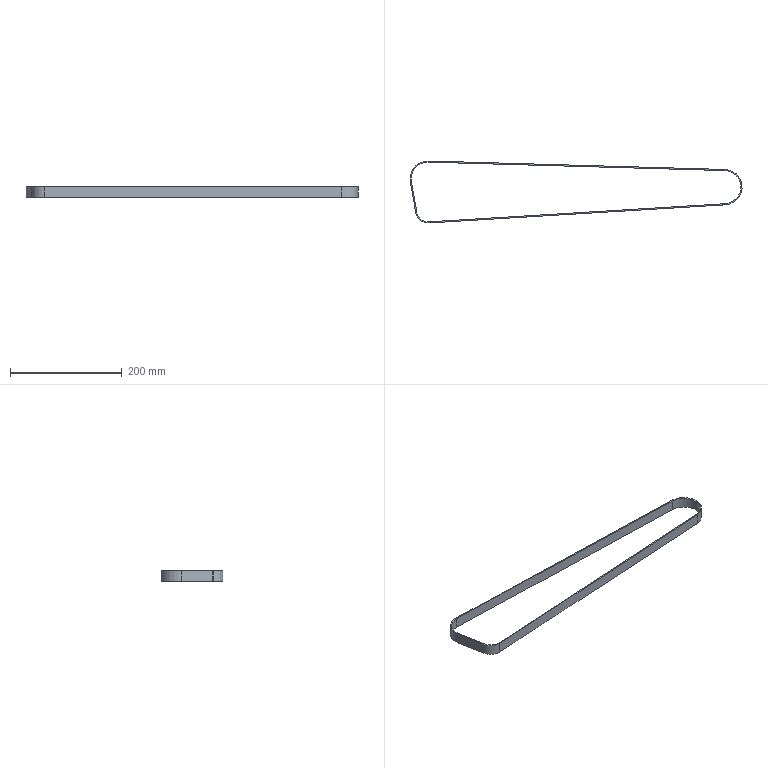Part | SolidWorks | features BaseBody 1 | 1 solid | 14 faces | box 593.838 x 110.876 x 19.05 mm | volume 50225 mm3 | plane 8 | cylinder 6 | commonest cylinder face diameters 59.266 x2 63.33 x2 39.054 x1 43.118 x1
STEP:
#1=CARTESIAN_POINT('',(532.317,-44.647,9.525));
#2=VERTEX_POINT('',#1);
#3=CARTESIAN_POINT('',(532.317,-44.647,-9.525));
#4=VERTEX_POINT('',#3);
#5=CARTESIAN_POINT('',(532.317,-44.647,9.525));
#6=DIRECTION('',(0.,0.,-1.));
#7=VECTOR('',#6,1000.);
#8=LINE('',#5,#7);
#9=EDGE_CURVE('',#2,#4,#8,.T.);
#10=ORIENTED_EDGE('',*,*,#9,.F.);
#11=CARTESIAN_POINT('',(531.349,14.552,9.525));
#12=VERTEX_POINT('',#11);
#13=CARTESIAN_POINT('',(530.507,-15.069,9.525));
#14=DIRECTION('',(0.,0.,-1.));
#15=DIRECTION('',(-0.06107,0.9981,0.));
#16=AXIS2_PLACEMENT_3D('',#13,#14,#15);
#17=CIRCLE('',#16,29.633);
#18=EDGE_CURVE('',#12,#2,#17,.T.);
#19=ORIENTED_EDGE('',*,*,#18,.F.);
#20=CARTESIAN_POINT('',(531.349,14.552,-9.525));
#21=VERTEX_POINT('',#20);
#22=CARTESIAN_POINT('',(531.349,14.552,9.525));
#23=DIRECTION('',(0.,0.,1.));
#24=VECTOR('',#23,1000.);
#25=LINE('',#22,#24);
#26=EDGE_CURVE('',#21,#12,#25,.T.);
#27=ORIENTED_EDGE('',*,*,#26,.F.);
#28=CARTESIAN_POINT('',(530.507,-15.069,-9.525));
#29=DIRECTION('',(0.,0.,-1.));
#30=DIRECTION('',(-0.06107,0.9981,0.));
#31=AXIS2_PLACEMENT_3D('',#28,#29,#30);
#32=CIRCLE('',#31,29.633);
#33=EDGE_CURVE('',#21,#4,#32,.T.);
#34=ORIENTED_EDGE('',*,*,#33,.T.);
#35=EDGE_LOOP('',(#10,#19,#27,#34));
#36=FACE_OUTER_BOUND('',#35,.T.);
#37=CARTESIAN_POINT('',(530.507,-15.069,0.));
#38=DIRECTION('',(0.,0.,1.));
#39=DIRECTION('',(-0.06107,0.9981,0.));
#40=AXIS2_PLACEMENT_3D('',#37,#38,#39);
#41=CYLINDRICAL_SURFACE('',#40,29.633);
#42=ADVANCED_FACE('',(#36),#41,.F.);
#43=CARTESIAN_POINT('',(532.441,-46.675,-9.525));
#44=VERTEX_POINT('',#43);
#45=CARTESIAN_POINT('',(532.441,-46.675,9.525));
#46=VERTEX_POINT('',#45);
#47=CARTESIAN_POINT('',(532.441,-46.675,-9.525));
#48=DIRECTION('',(0.,0.,1.));
#49=VECTOR('',#48,1000.);
#50=LINE('',#47,#49);
#51=EDGE_CURVE('',#44,#46,#50,.T.);
#52=ORIENTED_EDGE('',*,*,#51,.F.);
#53=CARTESIAN_POINT('',(531.406,16.584,-9.525));
#54=VERTEX_POINT('',#53);
#55=CARTESIAN_POINT('',(530.507,-15.069,-9.525));
#56=DIRECTION('',(0.,0.,-1.));
#57=DIRECTION('',(-0.06107,0.9981,0.));
#58=AXIS2_PLACEMENT_3D('',#55,#56,#57);
#59=CIRCLE('',#58,31.665);
#60=EDGE_CURVE('',#54,#44,#59,.T.);
#61=ORIENTED_EDGE('',*,*,#60,.F.);
#62=CARTESIAN_POINT('',(531.406,16.584,9.525));
#63=VERTEX_POINT('',#62);
#64=CARTESIAN_POINT('',(531.406,16.584,-9.525));
#65=DIRECTION('',(0.,0.,-1.));
#66=VECTOR('',#65,1000.);
#67=LINE('',#64,#66);
#68=EDGE_CURVE('',#63,#54,#67,.T.);
#69=ORIENTED_EDGE('',*,*,#68,.F.);
#70=CARTESIAN_POINT('',(530.507,-15.069,9.525));
#71=DIRECTION('',(0.,0.,-1.));
#72=DIRECTION('',(-0.06107,0.9981,0.));
#73=AXIS2_PLACEMENT_3D('',#70,#71,#72);
#74=CIRCLE('',#73,31.665);
#75=EDGE_CURVE('',#63,#46,#74,.T.);
#76=ORIENTED_EDGE('',*,*,#75,.T.);
#77=EDGE_LOOP('',(#52,#61,#69,#76));
#78=FACE_OUTER_BOUND('',#77,.T.);
#79=CARTESIAN_POINT('',(530.507,-15.069,0.));
#80=DIRECTION('',(0.,0.,1.));
#81=DIRECTION('',(-0.06107,0.9981,0.));
#82=AXIS2_PLACEMENT_3D('',#79,#80,#81);
#83=CYLINDRICAL_SURFACE('',#82,31.665);
#84=ADVANCED_FACE('',(#78),#83,.T.);
#85=ORIENTED_EDGE('',*,*,#26,.T.);
#86=CARTESIAN_POINT('',(0.8414,29.621,9.525));
#87=VERTEX_POINT('',#86);
#88=CARTESIAN_POINT('',(0.8414,29.621,9.525));
#89=DIRECTION('',(0.9996,-0.02839,0.));
#90=VECTOR('',#89,1000.);
#91=LINE('',#88,#90);
#92=EDGE_CURVE('',#87,#12,#91,.T.);
#93=ORIENTED_EDGE('',*,*,#92,.F.);
#94=CARTESIAN_POINT('',(0.8414,29.621,-9.525));
#95=VERTEX_POINT('',#94);
#96=CARTESIAN_POINT('',(0.8414,29.621,9.525));
#97=DIRECTION('',(0.,0.,1.));
#98=VECTOR('',#97,1000.);
#99=LINE('',#96,#98);
#100=EDGE_CURVE('',#95,#87,#99,.T.);
#101=ORIENTED_EDGE('',*,*,#100,.F.);
#102=CARTESIAN_POINT('',(0.8414,29.621,-9.525));
#103=DIRECTION('',(0.9996,-0.02839,0.));
#104=VECTOR('',#103,1000.);
#105=LINE('',#102,#104);
#106=EDGE_CURVE('',#95,#21,#105,.T.);
#107=ORIENTED_EDGE('',*,*,#106,.T.);
#108=EDGE_LOOP('',(#85,#93,#101,#107));
#109=FACE_OUTER_BOUND('',#108,.T.);
#110=CARTESIAN_POINT('',(0.8414,29.621,-9.525));
#111=DIRECTION('',(-0.02839,-0.9996,0.));
#112=DIRECTION('',(-0.9996,0.02839,0.));
#113=AXIS2_PLACEMENT_3D('',#110,#111,#112);
#114=PLANE('',#113);
#115=ADVANCED_FACE('',(#109),#114,.T.);
#116=ORIENTED_EDGE('',*,*,#68,.T.);
#117=CARTESIAN_POINT('',(0.8991,31.652,-9.525));
#118=VERTEX_POINT('',#117);
#119=CARTESIAN_POINT('',(0.8991,31.652,-9.525));
#120=DIRECTION('',(0.9996,-0.02839,0.));
#121=VECTOR('',#120,1000.);
#122=LINE('',#119,#121);
#123=EDGE_CURVE('',#118,#54,#122,.T.);
#124=ORIENTED_EDGE('',*,*,#123,.F.);
#125=CARTESIAN_POINT('',(0.8991,31.652,9.525));
#126=VERTEX_POINT('',#125);
#127=CARTESIAN_POINT('',(0.8991,31.652,-9.525));
#128=DIRECTION('',(0.,0.,-1.));
#129=VECTOR('',#128,1000.);
#130=LINE('',#127,#129);
#131=EDGE_CURVE('',#126,#118,#130,.T.);
#132=ORIENTED_EDGE('',*,*,#131,.F.);
#133=CARTESIAN_POINT('',(0.8991,31.652,9.525));
#134=DIRECTION('',(0.9996,-0.02839,0.));
#135=VECTOR('',#134,1000.);
#136=LINE('',#133,#135);
#137=EDGE_CURVE('',#126,#63,#136,.T.);
#138=ORIENTED_EDGE('',*,*,#137,.T.);
#139=EDGE_LOOP('',(#116,#124,#132,#138));
#140=FACE_OUTER_BOUND('',#139,.T.);
#141=CARTESIAN_POINT('',(0.8991,31.652,9.525));
#142=DIRECTION('',(0.02839,0.9996,0.));
#143=DIRECTION('',(0.,0.,-1.));
#144=AXIS2_PLACEMENT_3D('',#141,#142,#143);
#145=PLANE('',#144);
#146=ADVANCED_FACE('',(#140),#145,.T.);
#147=ORIENTED_EDGE('',*,*,#100,.T.);
#148=CARTESIAN_POINT('',(-29.176,-5.186,9.525));
#149=VERTEX_POINT('',#148);
#150=CARTESIAN_POINT('',(0.,0.,9.525));
#151=DIRECTION('',(0.,0.,-1.));
#152=DIRECTION('',(-0.02839,-0.9996,0.));
#153=AXIS2_PLACEMENT_3D('',#150,#151,#152);
#154=CIRCLE('',#153,29.633);
#155=EDGE_CURVE('',#149,#87,#154,.T.);
#156=ORIENTED_EDGE('',*,*,#155,.F.);
#157=CARTESIAN_POINT('',(-29.176,-5.186,-9.525));
#158=VERTEX_POINT('',#157);
#159=CARTESIAN_POINT('',(-29.176,-5.186,9.525));
#160=DIRECTION('',(0.,0.,1.));
#161=VECTOR('',#160,1000.);
#162=LINE('',#159,#161);
#163=EDGE_CURVE('',#158,#149,#162,.T.);
#164=ORIENTED_EDGE('',*,*,#163,.F.);
#165=CARTESIAN_POINT('',(0.,0.,-9.525));
#166=DIRECTION('',(0.,0.,-1.));
#167=DIRECTION('',(-0.02839,-0.9996,0.));
#168=AXIS2_PLACEMENT_3D('',#165,#166,#167);
#169=CIRCLE('',#168,29.633);
#170=EDGE_CURVE('',#158,#95,#169,.T.);
#171=ORIENTED_EDGE('',*,*,#170,.T.);
#172=EDGE_LOOP('',(#147,#156,#164,#171));
#173=FACE_OUTER_BOUND('',#172,.T.);
#174=CARTESIAN_POINT('',(0.,0.,0.));
#175=DIRECTION('',(0.,0.,1.));
#176=DIRECTION('',(-0.02839,-0.9996,0.));
#177=AXIS2_PLACEMENT_3D('',#174,#175,#176);
#178=CYLINDRICAL_SURFACE('',#177,29.633);
#179=ADVANCED_FACE('',(#173),#178,.F.);
#180=ORIENTED_EDGE('',*,*,#131,.T.);
#181=CARTESIAN_POINT('',(-31.176,-5.542,-9.525));
#182=VERTEX_POINT('',#181);
#183=CARTESIAN_POINT('',(0.,0.,-9.525));
#184=DIRECTION('',(0.,0.,-1.));
#185=DIRECTION('',(-0.02839,-0.9996,0.));
#186=AXIS2_PLACEMENT_3D('',#183,#184,#185);
#187=CIRCLE('',#186,31.665);
#188=EDGE_CURVE('',#182,#118,#187,.T.);
#189=ORIENTED_EDGE('',*,*,#188,.F.);
#190=CARTESIAN_POINT('',(-31.176,-5.542,9.525));
#191=VERTEX_POINT('',#190);
#192=CARTESIAN_POINT('',(-31.176,-5.542,-9.525));
#193=DIRECTION('',(0.,0.,-1.));
#194=VECTOR('',#193,1000.);
#195=LINE('',#192,#194);
#196=EDGE_CURVE('',#191,#182,#195,.T.);
#197=ORIENTED_EDGE('',*,*,#196,.F.);
#198=CARTESIAN_POINT('',(0.,0.,9.525));
#199=DIRECTION('',(0.,0.,-1.));
#200=DIRECTION('',(-0.02839,-0.9996,0.));
#201=AXIS2_PLACEMENT_3D('',#198,#199,#200);
#202=CIRCLE('',#201,31.665);
#203=EDGE_CURVE('',#191,#126,#202,.T.);
#204=ORIENTED_EDGE('',*,*,#203,.T.);
#205=EDGE_LOOP('',(#180,#189,#197,#204));
#206=FACE_OUTER_BOUND('',#205,.T.);
#207=CARTESIAN_POINT('',(0.,0.,0.));
#208=DIRECTION('',(0.,0.,1.));
#209=DIRECTION('',(-0.02839,-0.9996,0.));
#210=AXIS2_PLACEMENT_3D('',#207,#208,#209);
#211=CYLINDRICAL_SURFACE('',#210,31.665);
#212=ADVANCED_FACE('',(#206),#211,.T.);
#213=ORIENTED_EDGE('',*,*,#163,.T.);
#214=CARTESIAN_POINT('',(-19.242,-61.07,9.525));
#215=VERTEX_POINT('',#214);
#216=CARTESIAN_POINT('',(-19.242,-61.07,9.525));
#217=DIRECTION('',(-0.175,0.9846,0.));
#218=VECTOR('',#217,1000.);
#219=LINE('',#216,#218);
#220=EDGE_CURVE('',#215,#149,#219,.T.);
#221=ORIENTED_EDGE('',*,*,#220,.F.);
#222=CARTESIAN_POINT('',(-19.242,-61.07,-9.525));
#223=VERTEX_POINT('',#222);
#224=CARTESIAN_POINT('',(-19.242,-61.07,9.525));
#225=DIRECTION('',(0.,0.,1.));
#226=VECTOR('',#225,1000.);
#227=LINE('',#224,#226);
#228=EDGE_CURVE('',#223,#215,#227,.T.);
#229=ORIENTED_EDGE('',*,*,#228,.F.);
#230=CARTESIAN_POINT('',(-19.242,-61.07,-9.525));
#231=DIRECTION('',(-0.175,0.9846,0.));
#232=VECTOR('',#231,1000.);
#233=LINE('',#230,#232);
#234=EDGE_CURVE('',#223,#158,#233,.T.);
#235=ORIENTED_EDGE('',*,*,#234,.T.);
#236=EDGE_LOOP('',(#213,#221,#229,#235));
#237=FACE_OUTER_BOUND('',#236,.T.);
#238=CARTESIAN_POINT('',(-19.242,-61.07,-9.525));
#239=DIRECTION('',(0.9846,0.175,0.));
#240=DIRECTION('',(0.,0.,-1.));
#241=AXIS2_PLACEMENT_3D('',#238,#239,#240);
#242=PLANE('',#241);
#243=ADVANCED_FACE('',(#237),#242,.T.);
#244=ORIENTED_EDGE('',*,*,#196,.T.);
#245=CARTESIAN_POINT('',(-21.242,-61.425,-9.525));
#246=VERTEX_POINT('',#245);
#247=CARTESIAN_POINT('',(-21.242,-61.425,-9.525));
#248=DIRECTION('',(-0.175,0.9846,0.));
#249=VECTOR('',#248,1000.);
#250=LINE('',#247,#249);
#251=EDGE_CURVE('',#246,#182,#250,.T.);
#252=ORIENTED_EDGE('',*,*,#251,.F.);
#253=CARTESIAN_POINT('',(-21.242,-61.425,9.525));
#254=VERTEX_POINT('',#253);
#255=CARTESIAN_POINT('',(-21.242,-61.425,-9.525));
#256=DIRECTION('',(0.,0.,-1.));
#257=VECTOR('',#256,1000.);
#258=LINE('',#255,#257);
#259=EDGE_CURVE('',#254,#246,#258,.T.);
#260=ORIENTED_EDGE('',*,*,#259,.F.);
#261=CARTESIAN_POINT('',(-21.242,-61.425,9.525));
#262=DIRECTION('',(-0.175,0.9846,0.));
#263=VECTOR('',#262,1000.);
#264=LINE('',#261,#263);
#265=EDGE_CURVE('',#254,#191,#264,.T.);
#266=ORIENTED_EDGE('',*,*,#265,.T.);
#267=EDGE_LOOP('',(#244,#252,#260,#266));
#268=FACE_OUTER_BOUND('',#267,.T.);
#269=CARTESIAN_POINT('',(-21.242,-61.425,9.525));
#270=DIRECTION('',(-0.9846,-0.175,0.));
#271=DIRECTION('',(-0.175,0.9846,0.));
#272=AXIS2_PLACEMENT_3D('',#269,#270,#271);
#273=PLANE('',#272);
#274=ADVANCED_FACE('',(#268),#273,.T.);
#275=CARTESIAN_POINT('',(1.176,-77.143,-9.525));
#276=VERTEX_POINT('',#275);
#277=CARTESIAN_POINT('',(532.317,-44.647,-9.525));
#278=DIRECTION('',(-0.9981,-0.06107,0.));
#279=VECTOR('',#278,1000.);
#280=LINE('',#277,#279);
#281=EDGE_CURVE('',#4,#276,#280,.T.);
#282=ORIENTED_EDGE('',*,*,#281,.F.);
#283=ORIENTED_EDGE('',*,*,#33,.F.);
#284=ORIENTED_EDGE('',*,*,#106,.F.);
#285=ORIENTED_EDGE('',*,*,#170,.F.);
#286=ORIENTED_EDGE('',*,*,#234,.F.);
#287=CARTESIAN_POINT('',(-0.01632,-57.652,-9.525));
#288=DIRECTION('',(0.,0.,-1.));
#289=DIRECTION('',(0.9846,0.175,0.));
#290=AXIS2_PLACEMENT_3D('',#287,#288,#289);
#291=CIRCLE('',#290,19.527);
#292=EDGE_CURVE('',#276,#223,#291,.T.);
#293=ORIENTED_EDGE('',*,*,#292,.F.);
#294=EDGE_LOOP('',(#282,#283,#284,#285,#286,#293));
#295=FACE_BOUND('',#294,.T.);
#296=CARTESIAN_POINT('',(1.3,-79.171,-9.525));
#297=VERTEX_POINT('',#296);
#298=CARTESIAN_POINT('',(-0.01632,-57.652,-9.525));
#299=DIRECTION('',(0.,0.,-1.));
#300=DIRECTION('',(0.9846,0.175,0.));
#301=AXIS2_PLACEMENT_3D('',#298,#299,#300);
#302=CIRCLE('',#301,21.559);
#303=EDGE_CURVE('',#297,#246,#302,.T.);
#304=ORIENTED_EDGE('',*,*,#303,.T.);
#305=ORIENTED_EDGE('',*,*,#251,.T.);
#306=ORIENTED_EDGE('',*,*,#188,.T.);
#307=ORIENTED_EDGE('',*,*,#123,.T.);
#308=ORIENTED_EDGE('',*,*,#60,.T.);
#309=CARTESIAN_POINT('',(532.441,-46.675,-9.525));
#310=DIRECTION('',(-0.9981,-0.06107,0.));
#311=VECTOR('',#310,1000.);
#312=LINE('',#309,#311);
#313=EDGE_CURVE('',#44,#297,#312,.T.);
#314=ORIENTED_EDGE('',*,*,#313,.T.);
#315=EDGE_LOOP('',(#304,#305,#306,#307,#308,#314));
#316=FACE_OUTER_BOUND('',#315,.T.);
#317=CARTESIAN_POINT('',(1.238,-78.157,-9.525));
#318=DIRECTION('',(0.,0.,-1.));
#319=DIRECTION('',(0.,-1.,0.));
#320=AXIS2_PLACEMENT_3D('',#317,#318,#319);
#321=PLANE('',#320);
#322=ADVANCED_FACE('',(#295,#316),#321,.T.);
#323=ORIENTED_EDGE('',*,*,#228,.T.);
#324=CARTESIAN_POINT('',(1.176,-77.143,9.525));
#325=VERTEX_POINT('',#324);
#326=CARTESIAN_POINT('',(-0.01632,-57.652,9.525));
#327=DIRECTION('',(0.,0.,-1.));
#328=DIRECTION('',(0.9846,0.175,0.));
#329=AXIS2_PLACEMENT_3D('',#326,#327,#328);
#330=CIRCLE('',#329,19.527);
#331=EDGE_CURVE('',#325,#215,#330,.T.);
#332=ORIENTED_EDGE('',*,*,#331,.F.);
#333=CARTESIAN_POINT('',(1.176,-77.143,9.525));
#334=DIRECTION('',(0.,0.,1.));
#335=VECTOR('',#334,1000.);
#336=LINE('',#333,#335);
#337=EDGE_CURVE('',#276,#325,#336,.T.);
#338=ORIENTED_EDGE('',*,*,#337,.F.);
#339=ORIENTED_EDGE('',*,*,#292,.T.);
#340=EDGE_LOOP('',(#323,#332,#338,#339));
#341=FACE_OUTER_BOUND('',#340,.T.);
#342=CARTESIAN_POINT('',(-0.01632,-57.652,0.));
#343=DIRECTION('',(0.,0.,1.));
#344=DIRECTION('',(0.9846,0.175,0.));
#345=AXIS2_PLACEMENT_3D('',#342,#343,#344);
#346=CYLINDRICAL_SURFACE('',#345,19.527);
#347=ADVANCED_FACE('',(#341),#346,.F.);
#348=ORIENTED_EDGE('',*,*,#331,.T.);
#349=ORIENTED_EDGE('',*,*,#220,.T.);
#350=ORIENTED_EDGE('',*,*,#155,.T.);
#351=ORIENTED_EDGE('',*,*,#92,.T.);
#352=ORIENTED_EDGE('',*,*,#18,.T.);
#353=CARTESIAN_POINT('',(532.317,-44.647,9.525));
#354=DIRECTION('',(-0.9981,-0.06107,0.));
#355=VECTOR('',#354,1000.);
#356=LINE('',#353,#355);
#357=EDGE_CURVE('',#2,#325,#356,.T.);
#358=ORIENTED_EDGE('',*,*,#357,.T.);
#359=EDGE_LOOP('',(#348,#349,#350,#351,#352,#358));
#360=FACE_BOUND('',#359,.T.);
#361=CARTESIAN_POINT('',(1.3,-79.171,9.525));
#362=VERTEX_POINT('',#361);
#363=CARTESIAN_POINT('',(532.441,-46.675,9.525));
#364=DIRECTION('',(-0.9981,-0.06107,0.));
#365=VECTOR('',#364,1000.);
#366=LINE('',#363,#365);
#367=EDGE_CURVE('',#46,#362,#366,.T.);
#368=ORIENTED_EDGE('',*,*,#367,.F.);
#369=ORIENTED_EDGE('',*,*,#75,.F.);
#370=ORIENTED_EDGE('',*,*,#137,.F.);
#371=ORIENTED_EDGE('',*,*,#203,.F.);
#372=ORIENTED_EDGE('',*,*,#265,.F.);
#373=CARTESIAN_POINT('',(-0.01632,-57.652,9.525));
#374=DIRECTION('',(0.,0.,-1.));
#375=DIRECTION('',(0.9846,0.175,0.));
#376=AXIS2_PLACEMENT_3D('',#373,#374,#375);
#377=CIRCLE('',#376,21.559);
#378=EDGE_CURVE('',#362,#254,#377,.T.);
#379=ORIENTED_EDGE('',*,*,#378,.F.);
#380=EDGE_LOOP('',(#368,#369,#370,#371,#372,#379));
#381=FACE_OUTER_BOUND('',#380,.T.);
#382=CARTESIAN_POINT('',(1.238,-78.157,9.525));
#383=DIRECTION('',(0.,0.,1.));
#384=DIRECTION('',(1.,0.,0.));
#385=AXIS2_PLACEMENT_3D('',#382,#383,#384);
#386=PLANE('',#385);
#387=ADVANCED_FACE('',(#360,#381),#386,.T.);
#388=ORIENTED_EDGE('',*,*,#259,.T.);
#389=ORIENTED_EDGE('',*,*,#303,.F.);
#390=CARTESIAN_POINT('',(1.3,-79.171,-9.525));
#391=DIRECTION('',(0.,0.,-1.));
#392=VECTOR('',#391,1000.);
#393=LINE('',#390,#392);
#394=EDGE_CURVE('',#362,#297,#393,.T.);
#395=ORIENTED_EDGE('',*,*,#394,.F.);
#396=ORIENTED_EDGE('',*,*,#378,.T.);
#397=EDGE_LOOP('',(#388,#389,#395,#396));
#398=FACE_OUTER_BOUND('',#397,.T.);
#399=CARTESIAN_POINT('',(-0.01632,-57.652,0.));
#400=DIRECTION('',(0.,0.,1.));
#401=DIRECTION('',(0.9846,0.175,0.));
#402=AXIS2_PLACEMENT_3D('',#399,#400,#401);
#403=CYLINDRICAL_SURFACE('',#402,21.559);
#404=ADVANCED_FACE('',(#398),#403,.T.);
#405=ORIENTED_EDGE('',*,*,#337,.T.);
#406=ORIENTED_EDGE('',*,*,#357,.F.);
#407=ORIENTED_EDGE('',*,*,#9,.T.);
#408=ORIENTED_EDGE('',*,*,#281,.T.);
#409=EDGE_LOOP('',(#405,#406,#407,#408));
#410=FACE_OUTER_BOUND('',#409,.T.);
#411=CARTESIAN_POINT('',(532.317,-44.647,-9.525));
#412=DIRECTION('',(-0.06107,0.9981,0.));
#413=DIRECTION('',(0.,0.,1.));
#414=AXIS2_PLACEMENT_3D('',#411,#412,#413);
#415=PLANE('',#414);
#416=ADVANCED_FACE('',(#410),#415,.T.);
#417=ORIENTED_EDGE('',*,*,#394,.T.);
#418=ORIENTED_EDGE('',*,*,#313,.F.);
#419=ORIENTED_EDGE('',*,*,#51,.T.);
#420=ORIENTED_EDGE('',*,*,#367,.T.);
#421=EDGE_LOOP('',(#417,#418,#419,#420));
#422=FACE_OUTER_BOUND('',#421,.T.);
#423=CARTESIAN_POINT('',(532.441,-46.675,9.525));
#424=DIRECTION('',(0.06107,-0.9981,0.));
#425=DIRECTION('',(0.,0.,-1.));
#426=AXIS2_PLACEMENT_3D('',#423,#424,#425);
#427=PLANE('',#426);
#428=ADVANCED_FACE('',(#422),#427,.T.);
#429=CLOSED_SHELL('',(#42,#84,#115,#146,#179,#212,#243,#274,#322,#347,#387,#404,#416,#428));
#430=MANIFOLD_SOLID_BREP('',#429);
#431=CARTESIAN_POINT('',(0.,0.,0.));
#432=DIRECTION('',(0.,0.,1.));
#433=DIRECTION('',(1.,0.,0.));
#434=AXIS2_PLACEMENT_3D('',#431,#432,#433);
#435=(LENGTH_UNIT()NAMED_UNIT(*)SI_UNIT(.MILLI.,.METRE.));
#436=UNCERTAINTY_MEASURE_WITH_UNIT(LENGTH_MEASURE(0.00001),#435,'','');
#437=(NAMED_UNIT(*)PLANE_ANGLE_UNIT()SI_UNIT($,.RADIAN.));
#438=(NAMED_UNIT(*)SI_UNIT($,.STERADIAN.)SOLID_ANGLE_UNIT());
#439=(GEOMETRIC_REPRESENTATION_CONTEXT(3)GLOBAL_UNCERTAINTY_ASSIGNED_CONTEXT((#436))GLOBAL_UNIT_ASSIGNED_CONTEXT((#435,#437,#438))REPRESENTATION_CONTEXT('',''));
#440=ADVANCED_BREP_SHAPE_REPRESENTATION('',(#430,#434),#439);